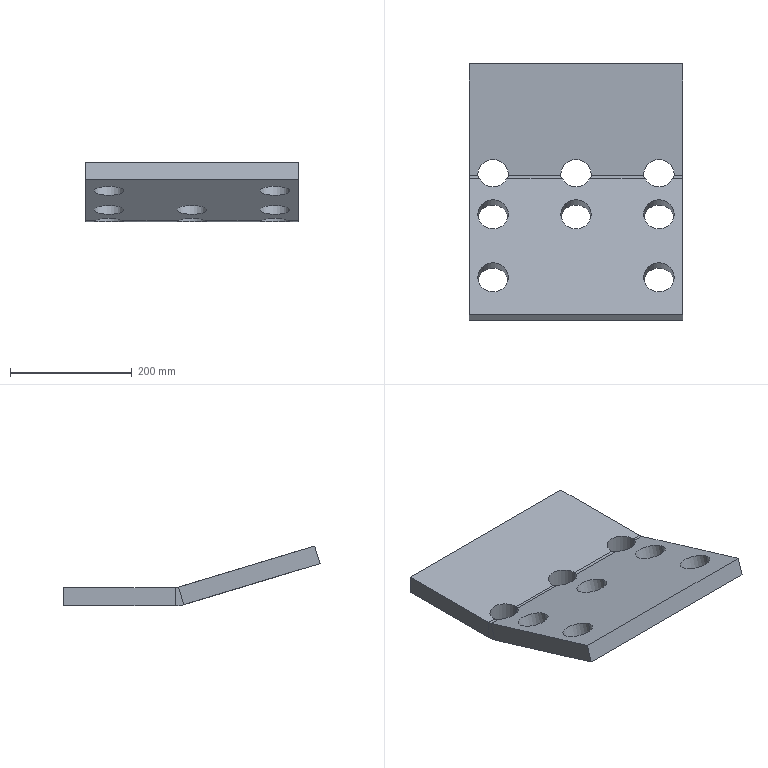Part | SolidWorks | features FlatPattern 1, SM3dBend 1, SMBaseFlange 1, SheetMetal 1 | 1 solid | 48 faces | box 350 x 419.833 x 98.276 mm | volume 3997529 mm3 | cylinder 30 | plane 12 | spline 6 | commonest cylinder face diameters 50 x22 40 x4 100 x4